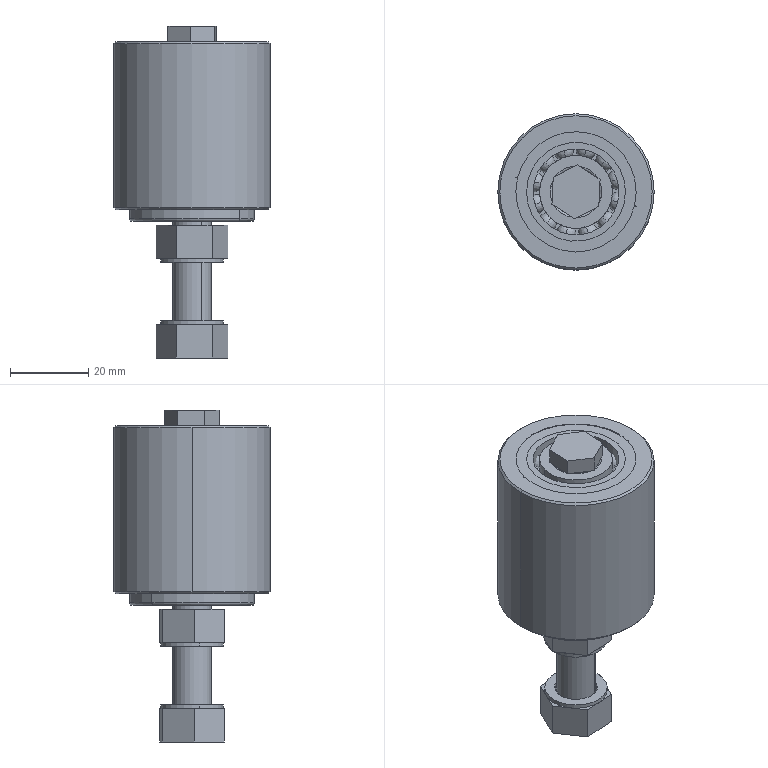Part | SolidWorks | 8 solids | 227 faces | box 40 x 40 x 85 mm | volume 60993 mm3 | torus 88 | sphere 48 | cylinder 46 | plane 41 | cone 4 | commonest cylinder face diameters 11 x8 18.667 x8 25.333 x8 16 x6 12 x4 22 x4